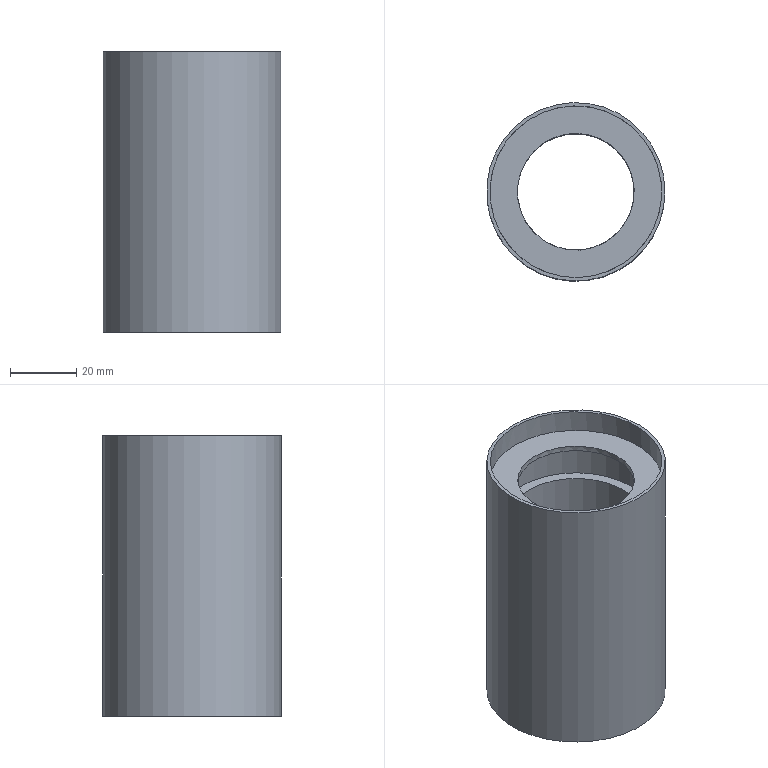Part | NX | features solid 2 | 1 solid | 16 faces | box 54.002 x 54.003 x 85.002 mm | volume 66964 mm3 | plane 8 | cylinder 8 | commonest cylinder face diameters 35.368 x2 46 x2 52 x2 40.028 x1 54 x1
STEP:
#1=CARTESIAN_POINT('',(-496.76,-938.893,-33.987));
#2=VERTEX_POINT('',#1);
#3=CARTESIAN_POINT('',(-484.114,-958.104,-33.986));
#4=DIRECTION('',(0.0000242,-0.00003327,-1.));
#5=DIRECTION('',(-0.5498,0.8353,-0.00004109));
#6=AXIS2_PLACEMENT_3D('',#3,#4,#5);
#7=CIRCLE('',#6,23.);
#8=EDGE_CURVE('',#2,#2,#7,.T.);
#9=ORIENTED_EDGE('',*,*,#8,.F.);
#10=EDGE_LOOP('',(#9));
#11=FACE_BOUND('',#10,.T.);
#12=CARTESIAN_POINT('',(-493.837,-943.333,-33.987));
#13=VERTEX_POINT('',#12);
#14=CARTESIAN_POINT('',(-484.114,-958.104,-33.986));
#15=DIRECTION('',(0.0000242,-0.00003327,-1.));
#16=DIRECTION('',(-0.5498,0.8353,-0.00004109));
#17=AXIS2_PLACEMENT_3D('',#14,#15,#16);
#18=CIRCLE('',#17,17.684);
#19=EDGE_CURVE('',#13,#13,#18,.T.);
#20=ORIENTED_EDGE('',*,*,#19,.T.);
#21=EDGE_LOOP('',(#20));
#22=FACE_BOUND('',#21,.T.);
#23=CARTESIAN_POINT('',(-501.654,-969.651,-33.986));
#24=DIRECTION('',(0.0000242,-0.00003327,-1.));
#25=DIRECTION('',(-0.5498,0.8353,-0.00004109));
#26=AXIS2_PLACEMENT_3D('',#23,#24,#25);
#27=PLANE('',#26);
#28=ADVANCED_FACE('',(#11,#22),#27,.F.);
#29=CARTESIAN_POINT('',(-496.76,-938.892,-21.987));
#30=VERTEX_POINT('',#29);
#31=CARTESIAN_POINT('',(-484.114,-958.104,-21.986));
#32=DIRECTION('',(0.0000242,-0.00003327,-1.));
#33=DIRECTION('',(-0.5498,0.8353,-0.00004109));
#34=AXIS2_PLACEMENT_3D('',#31,#32,#33);
#35=CIRCLE('',#34,23.);
#36=EDGE_CURVE('',#30,#30,#35,.T.);
#37=ORIENTED_EDGE('',*,*,#36,.F.);
#38=EDGE_LOOP('',(#37));
#39=FACE_BOUND('',#38,.T.);
#40=ORIENTED_EDGE('',*,*,#8,.T.);
#41=EDGE_LOOP('',(#40));
#42=FACE_BOUND('',#41,.T.);
#43=CARTESIAN_POINT('',(-484.116,-958.1,73.347));
#44=DIRECTION('',(0.0000242,-0.00003327,-1.));
#45=DIRECTION('',(-0.5498,0.8353,-0.00004109));
#46=AXIS2_PLACEMENT_3D('',#43,#44,#45);
#47=CYLINDRICAL_SURFACE('',#46,23.);
#48=ADVANCED_FACE('',(#39,#42),#47,.F.);
#49=CARTESIAN_POINT('',(-495.118,-941.387,-21.987));
#50=VERTEX_POINT('',#49);
#51=CARTESIAN_POINT('',(-484.114,-958.104,-21.986));
#52=DIRECTION('',(0.0000242,-0.00003327,-1.));
#53=DIRECTION('',(-0.5498,0.8353,-0.00004109));
#54=AXIS2_PLACEMENT_3D('',#51,#52,#53);
#55=CIRCLE('',#54,20.014);
#56=EDGE_CURVE('',#50,#50,#55,.T.);
#57=ORIENTED_EDGE('',*,*,#56,.F.);
#58=EDGE_LOOP('',(#57));
#59=FACE_BOUND('',#58,.T.);
#60=ORIENTED_EDGE('',*,*,#36,.T.);
#61=EDGE_LOOP('',(#60));
#62=FACE_BOUND('',#61,.T.);
#63=CARTESIAN_POINT('',(-503.325,-970.75,-21.986));
#64=DIRECTION('',(-0.0000242,0.00003327,1.));
#65=DIRECTION('',(0.5498,-0.8353,0.00004109));
#66=AXIS2_PLACEMENT_3D('',#63,#64,#65);
#67=PLANE('',#66);
#68=ADVANCED_FACE('',(#59,#62),#67,.F.);
#69=CARTESIAN_POINT('',(-495.119,-941.385,22.013));
#70=VERTEX_POINT('',#69);
#71=CARTESIAN_POINT('',(-484.115,-958.102,22.014));
#72=DIRECTION('',(0.0000242,-0.00003327,-1.));
#73=DIRECTION('',(-0.5498,0.8353,-0.00004109));
#74=AXIS2_PLACEMENT_3D('',#71,#72,#73);
#75=CIRCLE('',#74,20.014);
#76=EDGE_CURVE('',#70,#70,#75,.T.);
#77=ORIENTED_EDGE('',*,*,#76,.F.);
#78=EDGE_LOOP('',(#77));
#79=FACE_BOUND('',#78,.T.);
#80=ORIENTED_EDGE('',*,*,#56,.T.);
#81=EDGE_LOOP('',(#80));
#82=FACE_BOUND('',#81,.T.);
#83=CARTESIAN_POINT('',(-484.116,-958.1,73.347));
#84=DIRECTION('',(0.0000242,-0.00003327,-1.));
#85=DIRECTION('',(-0.5498,0.8353,-0.00004109));
#86=AXIS2_PLACEMENT_3D('',#83,#84,#85);
#87=CYLINDRICAL_SURFACE('',#86,20.014);
#88=ADVANCED_FACE('',(#79,#82),#87,.F.);
#89=CARTESIAN_POINT('',(-496.761,-938.891,22.013));
#90=VERTEX_POINT('',#89);
#91=CARTESIAN_POINT('',(-484.115,-958.102,22.014));
#92=DIRECTION('',(0.0000242,-0.00003327,-1.));
#93=DIRECTION('',(-0.5498,0.8353,-0.00004109));
#94=AXIS2_PLACEMENT_3D('',#91,#92,#93);
#95=CIRCLE('',#94,23.);
#96=EDGE_CURVE('',#90,#90,#95,.T.);
#97=ORIENTED_EDGE('',*,*,#96,.F.);
#98=EDGE_LOOP('',(#97));
#99=FACE_BOUND('',#98,.T.);
#100=ORIENTED_EDGE('',*,*,#76,.T.);
#101=EDGE_LOOP('',(#100));
#102=FACE_BOUND('',#101,.T.);
#103=CARTESIAN_POINT('',(-500.832,-969.107,22.014));
#104=DIRECTION('',(0.0000242,-0.00003327,-1.));
#105=DIRECTION('',(-0.5498,0.8353,-0.00004109));
#106=AXIS2_PLACEMENT_3D('',#103,#104,#105);
#107=PLANE('',#106);
#108=ADVANCED_FACE('',(#99,#102),#107,.F.);
#109=CARTESIAN_POINT('',(-496.762,-938.891,34.013));
#110=VERTEX_POINT('',#109);
#111=CARTESIAN_POINT('',(-484.115,-958.102,34.014));
#112=DIRECTION('',(0.0000242,-0.00003327,-1.));
#113=DIRECTION('',(-0.5498,0.8353,-0.00004109));
#114=AXIS2_PLACEMENT_3D('',#111,#112,#113);
#115=CIRCLE('',#114,23.);
#116=EDGE_CURVE('',#110,#110,#115,.T.);
#117=ORIENTED_EDGE('',*,*,#116,.F.);
#118=EDGE_LOOP('',(#117));
#119=FACE_BOUND('',#118,.T.);
#120=ORIENTED_EDGE('',*,*,#96,.T.);
#121=EDGE_LOOP('',(#120));
#122=FACE_BOUND('',#121,.T.);
#123=CARTESIAN_POINT('',(-484.116,-958.1,73.347));
#124=DIRECTION('',(0.0000242,-0.00003327,-1.));
#125=DIRECTION('',(-0.5498,0.8353,-0.00004109));
#126=AXIS2_PLACEMENT_3D('',#123,#124,#125);
#127=CYLINDRICAL_SURFACE('',#126,23.);
#128=ADVANCED_FACE('',(#119,#122),#127,.F.);
#129=CARTESIAN_POINT('',(-493.839,-943.331,34.013));
#130=VERTEX_POINT('',#129);
#131=CARTESIAN_POINT('',(-484.115,-958.102,34.014));
#132=DIRECTION('',(0.0000242,-0.00003327,-1.));
#133=DIRECTION('',(-0.5498,0.8353,-0.00004109));
#134=AXIS2_PLACEMENT_3D('',#131,#132,#133);
#135=CIRCLE('',#134,17.684);
#136=EDGE_CURVE('',#130,#130,#135,.T.);
#137=ORIENTED_EDGE('',*,*,#136,.F.);
#138=EDGE_LOOP('',(#137));
#139=FACE_BOUND('',#138,.T.);
#140=ORIENTED_EDGE('',*,*,#116,.T.);
#141=EDGE_LOOP('',(#140));
#142=FACE_BOUND('',#141,.T.);
#143=CARTESIAN_POINT('',(-501.656,-969.648,34.014));
#144=DIRECTION('',(-0.0000242,0.00003327,1.));
#145=DIRECTION('',(0.5498,-0.8353,0.00004109));
#146=AXIS2_PLACEMENT_3D('',#143,#144,#145);
#147=PLANE('',#146);
#148=ADVANCED_FACE('',(#139,#142),#147,.F.);
#149=CARTESIAN_POINT('',(-484.115,-940.418,35.614));
#150=VERTEX_POINT('',#149);
#151=CARTESIAN_POINT('',(-484.115,-958.102,35.614));
#152=DIRECTION('',(0.0000242,-0.00003327,-1.));
#153=DIRECTION('',(0.,1.,-0.00003327));
#154=AXIS2_PLACEMENT_3D('',#151,#152,#153);
#155=CIRCLE('',#154,17.684);
#156=EDGE_CURVE('',#150,#150,#155,.T.);
#157=ORIENTED_EDGE('',*,*,#156,.F.);
#158=EDGE_LOOP('',(#157));
#159=FACE_BOUND('',#158,.T.);
#160=ORIENTED_EDGE('',*,*,#136,.T.);
#161=EDGE_LOOP('',(#160));
#162=FACE_BOUND('',#161,.T.);
#163=CARTESIAN_POINT('',(-484.116,-958.1,73.347));
#164=DIRECTION('',(0.0000242,-0.00003327,-1.));
#165=DIRECTION('',(-0.5498,0.8353,-0.00004109));
#166=AXIS2_PLACEMENT_3D('',#163,#164,#165);
#167=CYLINDRICAL_SURFACE('',#166,17.684);
#168=ADVANCED_FACE('',(#159,#162),#167,.F.);
#169=CARTESIAN_POINT('',(-484.115,-932.102,35.613));
#170=VERTEX_POINT('',#169);
#171=CARTESIAN_POINT('',(-484.115,-958.102,35.614));
#172=DIRECTION('',(0.0000242,-0.00003327,-1.));
#173=DIRECTION('',(0.,1.,-0.00003327));
#174=AXIS2_PLACEMENT_3D('',#171,#172,#173);
#175=CIRCLE('',#174,26.);
#176=EDGE_CURVE('',#170,#170,#175,.T.);
#177=ORIENTED_EDGE('',*,*,#176,.F.);
#178=EDGE_LOOP('',(#177));
#179=FACE_BOUND('',#178,.T.);
#180=ORIENTED_EDGE('',*,*,#156,.T.);
#181=EDGE_LOOP('',(#180));
#182=FACE_BOUND('',#181,.T.);
#183=CARTESIAN_POINT('',(-498.886,-967.825,35.614));
#184=DIRECTION('',(0.0000242,-0.00003327,-1.));
#185=DIRECTION('',(-0.5498,0.8353,-0.00004109));
#186=AXIS2_PLACEMENT_3D('',#183,#184,#185);
#187=PLANE('',#186);
#188=ADVANCED_FACE('',(#179,#182),#187,.F.);
#189=CARTESIAN_POINT('',(-498.411,-936.385,42.513));
#190=VERTEX_POINT('',#189);
#191=CARTESIAN_POINT('',(-484.116,-958.102,42.514));
#192=DIRECTION('',(0.0000242,-0.00003327,-1.));
#193=DIRECTION('',(-0.5498,0.8353,-0.00004109));
#194=AXIS2_PLACEMENT_3D('',#191,#192,#193);
#195=CIRCLE('',#194,26.);
#196=EDGE_CURVE('',#190,#190,#195,.T.);
#197=ORIENTED_EDGE('',*,*,#196,.F.);
#198=EDGE_LOOP('',(#197));
#199=FACE_BOUND('',#198,.T.);
#200=ORIENTED_EDGE('',*,*,#176,.T.);
#201=EDGE_LOOP('',(#200));
#202=FACE_BOUND('',#201,.T.);
#203=CARTESIAN_POINT('',(-484.116,-958.1,73.347));
#204=DIRECTION('',(0.0000242,-0.00003327,-1.));
#205=DIRECTION('',(-0.5498,0.8353,-0.00004109));
#206=AXIS2_PLACEMENT_3D('',#203,#204,#205);
#207=CYLINDRICAL_SURFACE('',#206,26.);
#208=ADVANCED_FACE('',(#199,#202),#207,.F.);
#209=CARTESIAN_POINT('',(-498.961,-935.549,42.513));
#210=VERTEX_POINT('',#209);
#211=CARTESIAN_POINT('',(-484.116,-958.102,42.514));
#212=DIRECTION('',(0.0000242,-0.00003327,-1.));
#213=DIRECTION('',(-0.5498,0.8353,-0.00004109));
#214=AXIS2_PLACEMENT_3D('',#211,#212,#213);
#215=CIRCLE('',#214,27.);
#216=EDGE_CURVE('',#210,#210,#215,.T.);
#217=ORIENTED_EDGE('',*,*,#216,.F.);
#218=EDGE_LOOP('',(#217));
#219=FACE_BOUND('',#218,.T.);
#220=ORIENTED_EDGE('',*,*,#196,.T.);
#221=EDGE_LOOP('',(#220));
#222=FACE_BOUND('',#221,.T.);
#223=CARTESIAN_POINT('',(-505.833,-972.397,42.514));
#224=DIRECTION('',(0.0000242,-0.00003327,-1.));
#225=DIRECTION('',(-0.5498,0.8353,-0.00004109));
#226=AXIS2_PLACEMENT_3D('',#223,#224,#225);
#227=PLANE('',#226);
#228=ADVANCED_FACE('',(#219,#222),#227,.F.);
#229=CARTESIAN_POINT('',(-498.959,-935.552,-42.487));
#230=VERTEX_POINT('',#229);
#231=CARTESIAN_POINT('',(-484.113,-958.104,-42.486));
#232=DIRECTION('',(0.0000242,-0.00003327,-1.));
#233=DIRECTION('',(-0.5498,0.8353,-0.00004109));
#234=AXIS2_PLACEMENT_3D('',#231,#232,#233);
#235=CIRCLE('',#234,27.);
#236=EDGE_CURVE('',#230,#230,#235,.T.);
#237=ORIENTED_EDGE('',*,*,#236,.F.);
#238=EDGE_LOOP('',(#237));
#239=FACE_BOUND('',#238,.T.);
#240=ORIENTED_EDGE('',*,*,#216,.T.);
#241=EDGE_LOOP('',(#240));
#242=FACE_BOUND('',#241,.T.);
#243=CARTESIAN_POINT('',(-484.116,-958.1,73.347));
#244=DIRECTION('',(0.0000242,-0.00003327,-1.));
#245=DIRECTION('',(-0.5498,0.8353,-0.00004109));
#246=AXIS2_PLACEMENT_3D('',#243,#244,#245);
#247=CYLINDRICAL_SURFACE('',#246,27.);
#248=ADVANCED_FACE('',(#239,#242),#247,.T.);
#249=CARTESIAN_POINT('',(-498.409,-936.387,-42.487));
#250=VERTEX_POINT('',#249);
#251=CARTESIAN_POINT('',(-484.113,-958.104,-42.486));
#252=DIRECTION('',(0.0000242,-0.00003327,-1.));
#253=DIRECTION('',(-0.5498,0.8353,-0.00004109));
#254=AXIS2_PLACEMENT_3D('',#251,#252,#253);
#255=CIRCLE('',#254,26.);
#256=EDGE_CURVE('',#250,#250,#255,.T.);
#257=ORIENTED_EDGE('',*,*,#256,.F.);
#258=EDGE_LOOP('',(#257));
#259=FACE_BOUND('',#258,.T.);
#260=ORIENTED_EDGE('',*,*,#236,.T.);
#261=EDGE_LOOP('',(#260));
#262=FACE_BOUND('',#261,.T.);
#263=CARTESIAN_POINT('',(-506.666,-972.95,-42.486));
#264=DIRECTION('',(-0.0000242,0.00003327,1.));
#265=DIRECTION('',(0.5498,-0.8353,0.00004109));
#266=AXIS2_PLACEMENT_3D('',#263,#264,#265);
#267=PLANE('',#266);
#268=ADVANCED_FACE('',(#259,#262),#267,.F.);
#269=CARTESIAN_POINT('',(-484.114,-984.104,-35.585));
#270=VERTEX_POINT('',#269);
#271=CARTESIAN_POINT('',(-484.114,-958.104,-35.586));
#272=DIRECTION('',(-0.0000242,0.00003327,1.));
#273=DIRECTION('',(0.,-1.,0.00003327));
#274=AXIS2_PLACEMENT_3D('',#271,#272,#273);
#275=CIRCLE('',#274,26.);
#276=EDGE_CURVE('',#270,#270,#275,.F.);
#277=ORIENTED_EDGE('',*,*,#276,.F.);
#278=EDGE_LOOP('',(#277));
#279=FACE_BOUND('',#278,.T.);
#280=ORIENTED_EDGE('',*,*,#256,.T.);
#281=EDGE_LOOP('',(#280));
#282=FACE_BOUND('',#281,.T.);
#283=CARTESIAN_POINT('',(-484.116,-958.1,73.347));
#284=DIRECTION('',(0.0000242,-0.00003327,-1.));
#285=DIRECTION('',(-0.5498,0.8353,-0.00004109));
#286=AXIS2_PLACEMENT_3D('',#283,#284,#285);
#287=CYLINDRICAL_SURFACE('',#286,26.);
#288=ADVANCED_FACE('',(#279,#282),#287,.F.);
#289=CARTESIAN_POINT('',(-484.114,-975.788,-35.585));
#290=VERTEX_POINT('',#289);
#291=CARTESIAN_POINT('',(-484.114,-958.104,-35.586));
#292=DIRECTION('',(-0.0000242,0.00003327,1.));
#293=DIRECTION('',(0.,-1.,0.00003327));
#294=AXIS2_PLACEMENT_3D('',#291,#292,#293);
#295=CIRCLE('',#294,17.684);
#296=EDGE_CURVE('',#290,#290,#295,.F.);
#297=ORIENTED_EDGE('',*,*,#296,.F.);
#298=EDGE_LOOP('',(#297));
#299=FACE_BOUND('',#298,.T.);
#300=ORIENTED_EDGE('',*,*,#276,.T.);
#301=EDGE_LOOP('',(#300));
#302=FACE_BOUND('',#301,.T.);
#303=CARTESIAN_POINT('',(-505.831,-972.4,-35.586));
#304=DIRECTION('',(-0.0000242,0.00003327,1.));
#305=DIRECTION('',(0.5498,-0.8353,0.00004109));
#306=AXIS2_PLACEMENT_3D('',#303,#304,#305);
#307=PLANE('',#306);
#308=ADVANCED_FACE('',(#299,#302),#307,.F.);
#309=ORIENTED_EDGE('',*,*,#19,.F.);
#310=EDGE_LOOP('',(#309));
#311=FACE_BOUND('',#310,.T.);
#312=ORIENTED_EDGE('',*,*,#296,.T.);
#313=EDGE_LOOP('',(#312));
#314=FACE_BOUND('',#313,.T.);
#315=CARTESIAN_POINT('',(-484.116,-958.1,73.347));
#316=DIRECTION('',(0.0000242,-0.00003327,-1.));
#317=DIRECTION('',(-0.5498,0.8353,-0.00004109));
#318=AXIS2_PLACEMENT_3D('',#315,#316,#317);
#319=CYLINDRICAL_SURFACE('',#318,17.684);
#320=ADVANCED_FACE('',(#311,#314),#319,.F.);
#321=CLOSED_SHELL('',(#28,#48,#68,#88,#108,#128,#148,#168,#188,#208,#228,#248,#268,#288,#308,#320));
#322=MANIFOLD_SOLID_BREP('',#321);
#323=(LENGTH_UNIT()NAMED_UNIT(*)SI_UNIT(.MILLI.,.METRE.));
#324=UNCERTAINTY_MEASURE_WITH_UNIT(LENGTH_MEASURE(0.00001),#323,'','');
#325=(NAMED_UNIT(*)PLANE_ANGLE_UNIT()SI_UNIT($,.RADIAN.));
#326=(NAMED_UNIT(*)SI_UNIT($,.STERADIAN.)SOLID_ANGLE_UNIT());
#327=(GEOMETRIC_REPRESENTATION_CONTEXT(3)GLOBAL_UNCERTAINTY_ASSIGNED_CONTEXT((#324))GLOBAL_UNIT_ASSIGNED_CONTEXT((#323,#325,#326))REPRESENTATION_CONTEXT('',''));
#328=ADVANCED_BREP_SHAPE_REPRESENTATION('',(#322),#327);